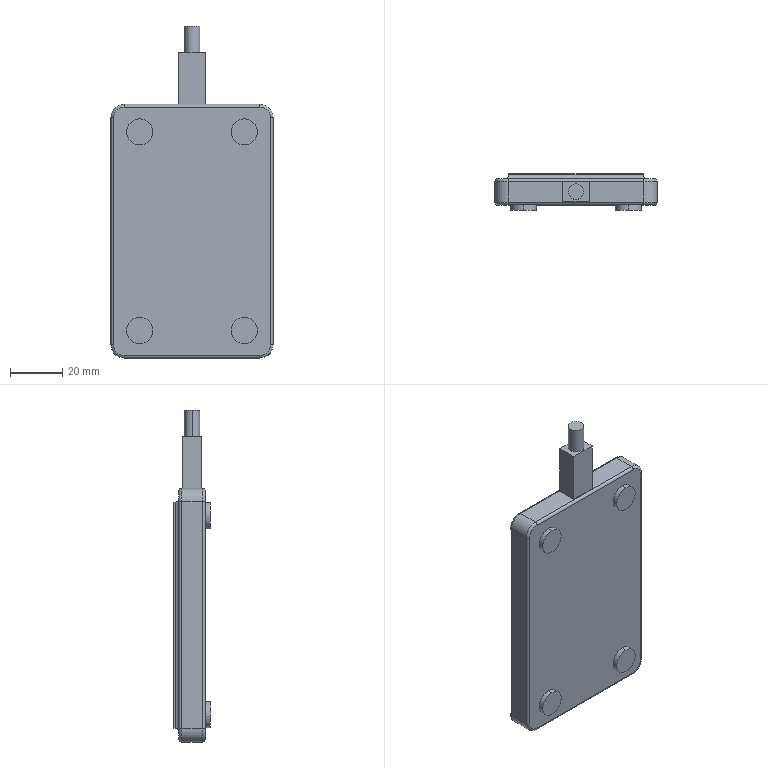Part | STEP file | Card reader | 1 solid | 64 faces | box 62 x 14 x 127 mm | volume 71225 mm3 | cylinder 30 | plane 26 | torus 8 | commonest cylinder face diameters 10 x12 2 x8 3 x4 4 x4 6 x2